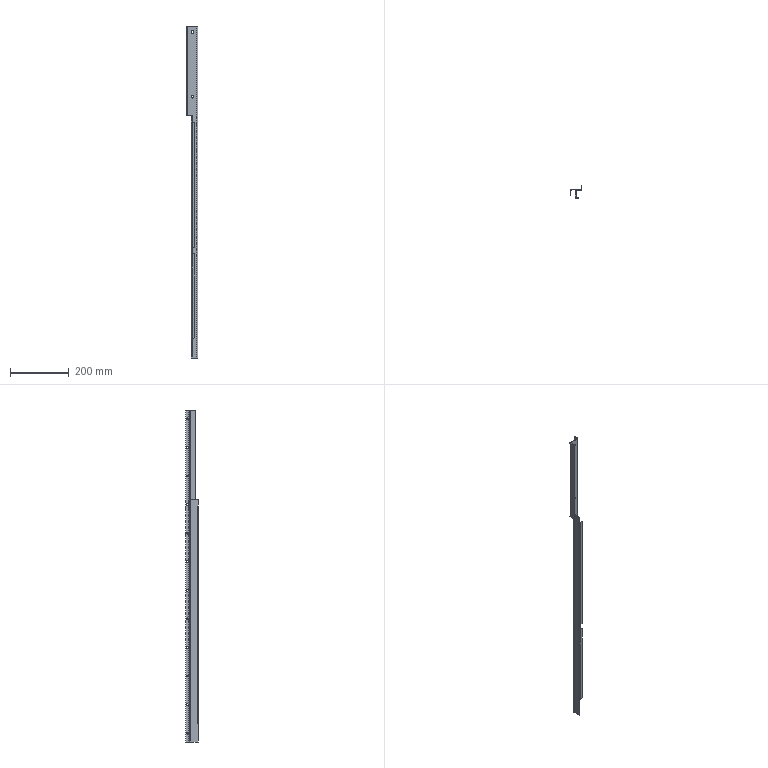Part | NX | features solid 2 | 1 solid | 72 faces | box 40 x 43 x 1127 mm | volume 153778 mm3 | cylinder 36 | plane 35 | spline 1 | commonest cylinder face diameters 6 x24 4 x4 8 x4 9.2 x4